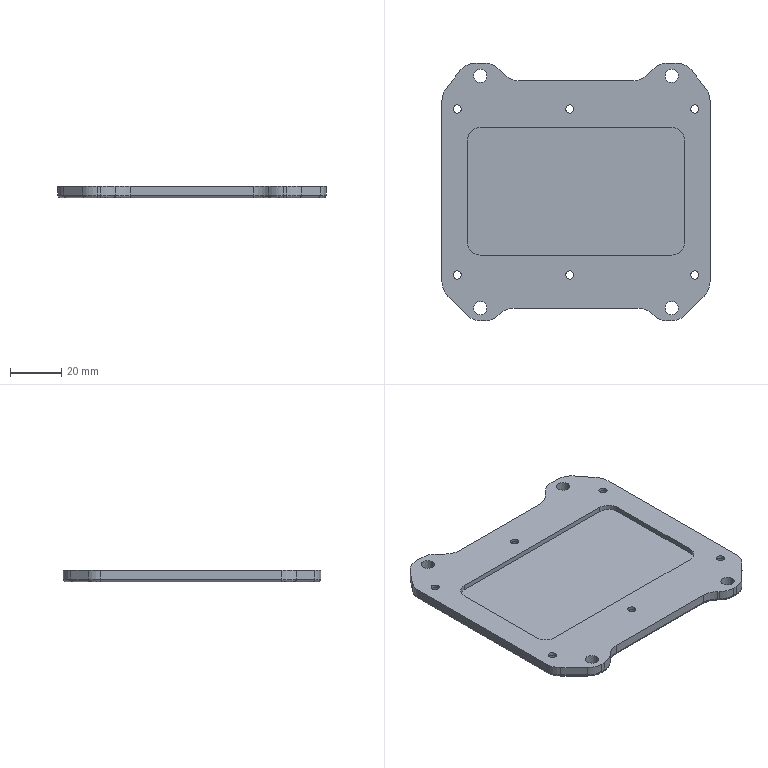NC program | NX | posted with a generic post | part box 105 x 101 x 4.5 mm
Lines 3938 to 3984 of 30641:
(PLANAR_MILL , TOOL : D8-25-D8-60-3T-FINISH)
N7844 T03 M6
N7846 G53
N7848 G17 G0 G90 X-23.408 Y-51.45 S3500 M3
N7850 G43 Z20. H3
N7852 Z-2.5
N7854 G94 G1 Z-5.5 F800.
N7856 X-24.222 Y-50.636
N7858 G3 X-27.05 Y-50.636 R2.
N7860 G1 X-27.364 Y-50.95
N7862 G2 X-35.814 Y-54.45 R11.95
N7864 G1 X-37.186
N7866 G2 X-45.636 Y-50.95 R11.95
N7868 G1 X-52.95 Y-43.636
N7870 G2 X-56.45 Y-35.186 R11.95
N7872 G1 Y35.734
N7874 G2 X-53.898 Y43.115 R11.95
N7876 G1 X-48.584 Y49.881
N7878 G2 X-39.186 Y54.45 R11.95
N7880 G1 X-35.814
N7882 G2 X-27.364 Y50.95 R11.95
N7884 G1 X-25.05 Y48.636
N7886 G3 X-22.186 Y47.45 R4.05
N7888 G1 X22.186
N7890 G3 X25.05 Y48.636 R4.05
N7892 G1 X27.364 Y50.95
N7894 G2 X35.814 Y54.45 R11.95
N7896 G1 X39.186
N7898 G2 X48.584 Y49.881 R11.95
N7900 G1 X53.898 Y43.115
N7902 G2 X56.45 Y35.734 R11.95
N7904 G1 Y-35.186
N7906 G2 X52.95 Y-43.636 R11.95
N7908 G1 X45.636 Y-50.95
N7910 G2 X37.186 Y-54.45 R11.95
N7912 G1 X35.814
N7914 G2 X27.364 Y-50.95 R11.95
N7916 G1 X27.05 Y-50.636
N7918 G3 X24.186 Y-49.45 R4.05
N7920 G1 X-24.186
N7922 G3 X-27.05 Y-50.636 R4.05
N7924 X-27.05 Y-53.465 R2.
N7926 G1 Z-2.5
N7928 G0 Z20.
N7930 M5